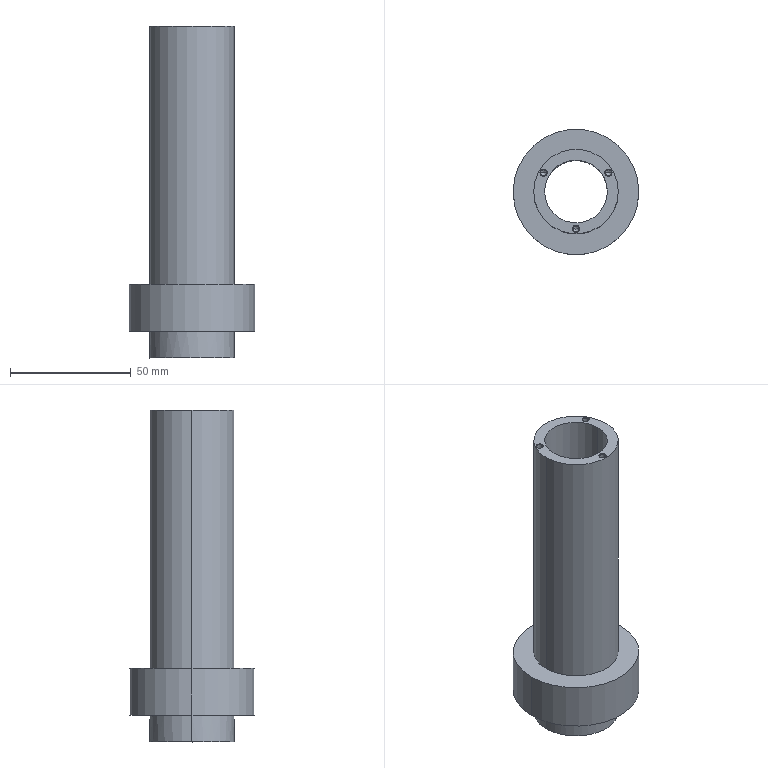Part | SolidWorks | features BaseBody 1 | 1 solid | 48 faces | box 52 x 52 x 137.45 mm | volume 81504 mm3 | cone 24 | cylinder 20 | plane 4 | commonest cylinder face diameters 2.5 x12 35 x4 26 x2 52 x2
STEP:
#1=CARTESIAN_POINT('',(359.676,258.457,27.673));
#2=VERTEX_POINT('',#1);
#3=CARTESIAN_POINT('',(360.758,257.832,26.922));
#4=VERTEX_POINT('',#3);
#5=CARTESIAN_POINT('',(360.287,258.104,27.249));
#6=DIRECTION('',(0.7423,-0.4286,-0.515));
#7=VECTOR('',#6,1000.);
#8=LINE('',#5,#7);
#9=EDGE_CURVE('',#2,#4,#8,.T.);
#10=ORIENTED_EDGE('',*,*,#9,.F.);
#11=CARTESIAN_POINT('',(358.593,259.082,26.922));
#12=VERTEX_POINT('',#11);
#13=CARTESIAN_POINT('',(359.065,258.81,27.249));
#14=DIRECTION('',(-0.7423,0.4286,-0.515));
#15=VECTOR('',#14,1000.);
#16=LINE('',#13,#15);
#17=EDGE_CURVE('',#2,#12,#16,.T.);
#18=ORIENTED_EDGE('',*,*,#17,.T.);
#19=CARTESIAN_POINT('',(359.676,258.457,26.922));
#20=DIRECTION('',(0.,0.,-1.));
#21=DIRECTION('',(0.866,-0.5,0.));
#22=AXIS2_PLACEMENT_3D('',#19,#20,#21);
#23=CIRCLE('',#22,1.25);
#24=EDGE_CURVE('',#12,#4,#23,.T.);
#25=ORIENTED_EDGE('',*,*,#24,.T.);
#26=EDGE_LOOP('',(#10,#18,#25));
#27=FACE_OUTER_BOUND('',#26,.T.);
#28=CARTESIAN_POINT('',(359.676,258.457,27.249));
#29=DIRECTION('',(0.,0.,-1.));
#30=DIRECTION('',(0.866,-0.5,0.));
#31=AXIS2_PLACEMENT_3D('',#28,#29,#30);
#32=CONICAL_SURFACE('',#31,0.7052,1.03);
#33=ADVANCED_FACE('',(#27),#32,.F.);
#34=CARTESIAN_POINT('',(360.758,257.832,15.721));
#35=VERTEX_POINT('',#34);
#36=CARTESIAN_POINT('',(360.301,259.54,15.721));
#37=VERTEX_POINT('',#36);
#38=CARTESIAN_POINT('',(359.676,258.457,15.721));
#39=DIRECTION('',(0.,0.,1.));
#40=DIRECTION('',(-0.866,0.5,0.));
#41=AXIS2_PLACEMENT_3D('',#38,#39,#40);
#42=CIRCLE('',#41,1.25);
#43=EDGE_CURVE('',#35,#37,#42,.T.);
#44=ORIENTED_EDGE('',*,*,#43,.F.);
#45=CARTESIAN_POINT('',(360.758,257.832,15.471));
#46=DIRECTION('',(0.,0.,1.));
#47=VECTOR('',#46,1000.);
#48=LINE('',#45,#47);
#49=EDGE_CURVE('',#35,#4,#48,.T.);
#50=ORIENTED_EDGE('',*,*,#49,.T.);
#51=ORIENTED_EDGE('',*,*,#24,.F.);
#52=CARTESIAN_POINT('',(358.593,259.082,15.721));
#53=VERTEX_POINT('',#52);
#54=CARTESIAN_POINT('',(358.593,259.082,15.471));
#55=DIRECTION('',(0.,0.,1.));
#56=VECTOR('',#55,1000.);
#57=LINE('',#54,#56);
#58=EDGE_CURVE('',#53,#12,#57,.T.);
#59=ORIENTED_EDGE('',*,*,#58,.F.);
#60=CARTESIAN_POINT('',(359.676,258.457,15.721));
#61=DIRECTION('',(0.,0.,1.));
#62=DIRECTION('',(-0.866,0.5,0.));
#63=AXIS2_PLACEMENT_3D('',#60,#61,#62);
#64=CIRCLE('',#63,1.25);
#65=EDGE_CURVE('',#37,#53,#64,.T.);
#66=ORIENTED_EDGE('',*,*,#65,.F.);
#67=EDGE_LOOP('',(#44,#50,#51,#59,#66));
#68=FACE_OUTER_BOUND('',#67,.T.);
#69=CARTESIAN_POINT('',(359.676,258.457,15.471));
#70=DIRECTION('',(0.,0.,1.));
#71=DIRECTION('',(-0.866,0.5,0.));
#72=AXIS2_PLACEMENT_3D('',#69,#70,#71);
#73=CYLINDRICAL_SURFACE('',#72,1.25);
#74=ADVANCED_FACE('',(#68),#73,.F.);
#75=ORIENTED_EDGE('',*,*,#65,.T.);
#76=CARTESIAN_POINT('',(359.051,257.375,15.721));
#77=VERTEX_POINT('',#76);
#78=CARTESIAN_POINT('',(359.676,258.457,15.721));
#79=DIRECTION('',(0.,0.,1.));
#80=DIRECTION('',(-0.866,0.5,0.));
#81=AXIS2_PLACEMENT_3D('',#78,#79,#80);
#82=CIRCLE('',#81,1.25);
#83=EDGE_CURVE('',#53,#77,#82,.T.);
#84=ORIENTED_EDGE('',*,*,#83,.T.);
#85=CARTESIAN_POINT('',(358.926,257.158,15.471));
#86=VERTEX_POINT('',#85);
#87=CARTESIAN_POINT('',(358.988,257.266,15.596));
#88=DIRECTION('',(-0.3536,-0.6124,-0.7071));
#89=VECTOR('',#88,1000.);
#90=LINE('',#87,#89);
#91=EDGE_CURVE('',#77,#86,#90,.T.);
#92=ORIENTED_EDGE('',*,*,#91,.T.);
#93=CARTESIAN_POINT('',(360.426,259.756,15.471));
#94=VERTEX_POINT('',#93);
#95=CARTESIAN_POINT('',(359.676,258.457,15.471));
#96=DIRECTION('',(0.,0.,1.));
#97=DIRECTION('',(0.866,-0.5,0.));
#98=AXIS2_PLACEMENT_3D('',#95,#96,#97);
#99=CIRCLE('',#98,1.5);
#100=EDGE_CURVE('',#94,#86,#99,.T.);
#101=ORIENTED_EDGE('',*,*,#100,.F.);
#102=CARTESIAN_POINT('',(360.363,259.648,15.596));
#103=DIRECTION('',(0.3536,0.6124,-0.7071));
#104=VECTOR('',#103,1000.);
#105=LINE('',#102,#104);
#106=EDGE_CURVE('',#37,#94,#105,.T.);
#107=ORIENTED_EDGE('',*,*,#106,.F.);
#108=EDGE_LOOP('',(#75,#84,#92,#101,#107));
#109=FACE_OUTER_BOUND('',#108,.T.);
#110=CARTESIAN_POINT('',(359.676,258.457,15.596));
#111=DIRECTION('',(0.,0.,-1.));
#112=DIRECTION('',(0.5,0.866,0.));
#113=AXIS2_PLACEMENT_3D('',#110,#111,#112);
#114=CONICAL_SURFACE('',#113,1.375,0.7854);
#115=ADVANCED_FACE('',(#109),#114,.F.);
#116=CARTESIAN_POINT('',(322.653,258.943,15.721));
#117=VERTEX_POINT('',#116);
#118=CARTESIAN_POINT('',(320.946,259.401,15.721));
#119=VERTEX_POINT('',#118);
#120=CARTESIAN_POINT('',(321.571,258.318,15.721));
#121=DIRECTION('',(0.,0.,1.));
#122=DIRECTION('',(-0.866,-0.5,0.));
#123=AXIS2_PLACEMENT_3D('',#120,#121,#122);
#124=CIRCLE('',#123,1.25);
#125=EDGE_CURVE('',#117,#119,#124,.T.);
#126=ORIENTED_EDGE('',*,*,#125,.T.);
#127=CARTESIAN_POINT('',(320.821,259.617,15.471));
#128=VERTEX_POINT('',#127);
#129=CARTESIAN_POINT('',(320.883,259.509,15.596));
#130=DIRECTION('',(-0.3536,0.6124,-0.7071));
#131=VECTOR('',#130,1000.);
#132=LINE('',#129,#131);
#133=EDGE_CURVE('',#119,#128,#132,.T.);
#134=ORIENTED_EDGE('',*,*,#133,.T.);
#135=CARTESIAN_POINT('',(322.321,257.019,15.471));
#136=VERTEX_POINT('',#135);
#137=CARTESIAN_POINT('',(321.571,258.318,15.471));
#138=DIRECTION('',(0.,0.,1.));
#139=DIRECTION('',(0.5,-0.866,0.));
#140=AXIS2_PLACEMENT_3D('',#137,#138,#139);
#141=CIRCLE('',#140,1.5);
#142=EDGE_CURVE('',#136,#128,#141,.T.);
#143=ORIENTED_EDGE('',*,*,#142,.F.);
#144=CARTESIAN_POINT('',(322.196,257.236,15.721));
#145=VERTEX_POINT('',#144);
#146=CARTESIAN_POINT('',(322.258,257.128,15.596));
#147=DIRECTION('',(0.3536,-0.6124,-0.7071));
#148=VECTOR('',#147,1000.);
#149=LINE('',#146,#148);
#150=EDGE_CURVE('',#145,#136,#149,.T.);
#151=ORIENTED_EDGE('',*,*,#150,.F.);
#152=CARTESIAN_POINT('',(321.571,258.318,15.721));
#153=DIRECTION('',(0.,0.,1.));
#154=DIRECTION('',(-0.866,-0.5,0.));
#155=AXIS2_PLACEMENT_3D('',#152,#153,#154);
#156=CIRCLE('',#155,1.25);
#157=EDGE_CURVE('',#145,#117,#156,.T.);
#158=ORIENTED_EDGE('',*,*,#157,.T.);
#159=EDGE_LOOP('',(#126,#134,#143,#151,#158));
#160=FACE_OUTER_BOUND('',#159,.T.);
#161=CARTESIAN_POINT('',(321.571,258.318,15.596));
#162=DIRECTION('',(0.,0.,-1.));
#163=DIRECTION('',(0.5,-0.866,0.));
#164=AXIS2_PLACEMENT_3D('',#161,#162,#163);
#165=CONICAL_SURFACE('',#164,1.375,0.7854);
#166=ADVANCED_FACE('',(#160),#165,.F.);
#167=CARTESIAN_POINT('',(320.488,257.693,15.721));
#168=VERTEX_POINT('',#167);
#169=CARTESIAN_POINT('',(321.571,258.318,15.721));
#170=DIRECTION('',(0.,0.,1.));
#171=DIRECTION('',(-0.866,-0.5,0.));
#172=AXIS2_PLACEMENT_3D('',#169,#170,#171);
#173=CIRCLE('',#172,1.25);
#174=EDGE_CURVE('',#168,#145,#173,.T.);
#175=ORIENTED_EDGE('',*,*,#174,.F.);
#176=CARTESIAN_POINT('',(320.488,257.693,26.922));
#177=VERTEX_POINT('',#176);
#178=CARTESIAN_POINT('',(320.488,257.693,15.471));
#179=DIRECTION('',(0.,0.,1.));
#180=VECTOR('',#179,1000.);
#181=LINE('',#178,#180);
#182=EDGE_CURVE('',#168,#177,#181,.T.);
#183=ORIENTED_EDGE('',*,*,#182,.T.);
#184=CARTESIAN_POINT('',(322.653,258.943,26.922));
#185=VERTEX_POINT('',#184);
#186=CARTESIAN_POINT('',(321.571,258.318,26.922));
#187=DIRECTION('',(0.,0.,-1.));
#188=DIRECTION('',(-0.866,-0.5,0.));
#189=AXIS2_PLACEMENT_3D('',#186,#187,#188);
#190=CIRCLE('',#189,1.25);
#191=EDGE_CURVE('',#185,#177,#190,.T.);
#192=ORIENTED_EDGE('',*,*,#191,.F.);
#193=CARTESIAN_POINT('',(322.653,258.943,15.471));
#194=DIRECTION('',(0.,0.,1.));
#195=VECTOR('',#194,1000.);
#196=LINE('',#193,#195);
#197=EDGE_CURVE('',#117,#185,#196,.T.);
#198=ORIENTED_EDGE('',*,*,#197,.F.);
#199=ORIENTED_EDGE('',*,*,#157,.F.);
#200=EDGE_LOOP('',(#175,#183,#192,#198,#199));
#201=FACE_OUTER_BOUND('',#200,.T.);
#202=CARTESIAN_POINT('',(321.571,258.318,15.471));
#203=DIRECTION('',(0.,0.,1.));
#204=DIRECTION('',(0.866,0.5,0.));
#205=AXIS2_PLACEMENT_3D('',#202,#203,#204);
#206=CYLINDRICAL_SURFACE('',#205,1.25);
#207=ADVANCED_FACE('',(#201),#206,.F.);
#208=CARTESIAN_POINT('',(321.571,258.318,27.673));
#209=VERTEX_POINT('',#208);
#210=CARTESIAN_POINT('',(320.96,257.966,27.249));
#211=DIRECTION('',(-0.7423,-0.4286,-0.515));
#212=VECTOR('',#211,1000.);
#213=LINE('',#210,#212);
#214=EDGE_CURVE('',#209,#177,#213,.T.);
#215=ORIENTED_EDGE('',*,*,#214,.F.);
#216=CARTESIAN_POINT('',(322.182,258.671,27.249));
#217=DIRECTION('',(0.7423,0.4286,-0.515));
#218=VECTOR('',#217,1000.);
#219=LINE('',#216,#218);
#220=EDGE_CURVE('',#209,#185,#219,.T.);
#221=ORIENTED_EDGE('',*,*,#220,.T.);
#222=ORIENTED_EDGE('',*,*,#191,.T.);
#223=EDGE_LOOP('',(#215,#221,#222));
#224=FACE_OUTER_BOUND('',#223,.T.);
#225=CARTESIAN_POINT('',(321.571,258.318,27.249));
#226=DIRECTION('',(0.,0.,-1.));
#227=DIRECTION('',(-0.866,-0.5,0.));
#228=AXIS2_PLACEMENT_3D('',#225,#226,#227);
#229=CONICAL_SURFACE('',#228,0.7052,1.03);
#230=ADVANCED_FACE('',(#224),#229,.F.);
#231=CARTESIAN_POINT('',(340.503,290.138,15.721));
#232=VERTEX_POINT('',#231);
#233=CARTESIAN_POINT('',(341.753,291.388,15.721));
#234=VERTEX_POINT('',#233);
#235=CARTESIAN_POINT('',(340.503,291.388,15.721));
#236=DIRECTION('',(0.,0.,1.));
#237=DIRECTION('',(0.,1.,0.));
#238=AXIS2_PLACEMENT_3D('',#235,#236,#237);
#239=CIRCLE('',#238,1.25);
#240=EDGE_CURVE('',#232,#234,#239,.T.);
#241=ORIENTED_EDGE('',*,*,#240,.T.);
#242=CARTESIAN_POINT('',(342.003,291.388,15.471));
#243=VERTEX_POINT('',#242);
#244=CARTESIAN_POINT('',(341.878,291.388,15.596));
#245=DIRECTION('',(0.7071,0.,-0.7071));
#246=VECTOR('',#245,1000.);
#247=LINE('',#244,#246);
#248=EDGE_CURVE('',#234,#243,#247,.T.);
#249=ORIENTED_EDGE('',*,*,#248,.T.);
#250=CARTESIAN_POINT('',(339.003,291.388,15.471));
#251=VERTEX_POINT('',#250);
#252=CARTESIAN_POINT('',(340.503,291.388,15.471));
#253=DIRECTION('',(0.,0.,1.));
#254=DIRECTION('',(-1.,0.,0.));
#255=AXIS2_PLACEMENT_3D('',#252,#253,#254);
#256=CIRCLE('',#255,1.5);
#257=EDGE_CURVE('',#251,#243,#256,.T.);
#258=ORIENTED_EDGE('',*,*,#257,.F.);
#259=CARTESIAN_POINT('',(339.253,291.388,15.721));
#260=VERTEX_POINT('',#259);
#261=CARTESIAN_POINT('',(339.128,291.388,15.596));
#262=DIRECTION('',(-0.7071,0.,-0.7071));
#263=VECTOR('',#262,1000.);
#264=LINE('',#261,#263);
#265=EDGE_CURVE('',#260,#251,#264,.T.);
#266=ORIENTED_EDGE('',*,*,#265,.F.);
#267=CARTESIAN_POINT('',(340.503,291.388,15.721));
#268=DIRECTION('',(0.,0.,1.));
#269=DIRECTION('',(0.,1.,0.));
#270=AXIS2_PLACEMENT_3D('',#267,#268,#269);
#271=CIRCLE('',#270,1.25);
#272=EDGE_CURVE('',#260,#232,#271,.T.);
#273=ORIENTED_EDGE('',*,*,#272,.T.);
#274=EDGE_LOOP('',(#241,#249,#258,#266,#273));
#275=FACE_OUTER_BOUND('',#274,.T.);
#276=CARTESIAN_POINT('',(340.503,291.388,15.596));
#277=DIRECTION('',(0.,0.,-1.));
#278=DIRECTION('',(-1.,0.,0.));
#279=AXIS2_PLACEMENT_3D('',#276,#277,#278);
#280=CONICAL_SURFACE('',#279,1.375,0.7854);
#281=ADVANCED_FACE('',(#275),#280,.F.);
#282=CARTESIAN_POINT('',(340.503,292.638,15.721));
#283=VERTEX_POINT('',#282);
#284=CARTESIAN_POINT('',(340.503,291.388,15.721));
#285=DIRECTION('',(0.,0.,1.));
#286=DIRECTION('',(0.,1.,0.));
#287=AXIS2_PLACEMENT_3D('',#284,#285,#286);
#288=CIRCLE('',#287,1.25);
#289=EDGE_CURVE('',#283,#260,#288,.T.);
#290=ORIENTED_EDGE('',*,*,#289,.F.);
#291=CARTESIAN_POINT('',(340.503,292.638,26.922));
#292=VERTEX_POINT('',#291);
#293=CARTESIAN_POINT('',(340.503,292.638,15.471));
#294=DIRECTION('',(0.,0.,1.));
#295=VECTOR('',#294,1000.);
#296=LINE('',#293,#295);
#297=EDGE_CURVE('',#283,#292,#296,.T.);
#298=ORIENTED_EDGE('',*,*,#297,.T.);
#299=CARTESIAN_POINT('',(340.503,290.138,26.922));
#300=VERTEX_POINT('',#299);
#301=CARTESIAN_POINT('',(340.503,291.388,26.922));
#302=DIRECTION('',(0.,0.,-1.));
#303=DIRECTION('',(0.,1.,0.));
#304=AXIS2_PLACEMENT_3D('',#301,#302,#303);
#305=CIRCLE('',#304,1.25);
#306=EDGE_CURVE('',#300,#292,#305,.T.);
#307=ORIENTED_EDGE('',*,*,#306,.F.);
#308=CARTESIAN_POINT('',(340.503,290.138,15.471));
#309=DIRECTION('',(0.,0.,1.));
#310=VECTOR('',#309,1000.);
#311=LINE('',#308,#310);
#312=EDGE_CURVE('',#232,#300,#311,.T.);
#313=ORIENTED_EDGE('',*,*,#312,.F.);
#314=ORIENTED_EDGE('',*,*,#272,.F.);
#315=EDGE_LOOP('',(#290,#298,#307,#313,#314));
#316=FACE_OUTER_BOUND('',#315,.T.);
#317=CARTESIAN_POINT('',(340.503,291.388,15.471));
#318=DIRECTION('',(0.,0.,1.));
#319=DIRECTION('',(0.,-1.,0.));
#320=AXIS2_PLACEMENT_3D('',#317,#318,#319);
#321=CYLINDRICAL_SURFACE('',#320,1.25);
#322=ADVANCED_FACE('',(#316),#321,.F.);
#323=CARTESIAN_POINT('',(340.503,291.388,27.673));
#324=VERTEX_POINT('',#323);
#325=CARTESIAN_POINT('',(340.503,292.093,27.249));
#326=DIRECTION('',(0.,0.8572,-0.515));
#327=VECTOR('',#326,1000.);
#328=LINE('',#325,#327);
#329=EDGE_CURVE('',#324,#292,#328,.T.);
#330=ORIENTED_EDGE('',*,*,#329,.F.);
#331=CARTESIAN_POINT('',(340.503,290.682,27.249));
#332=DIRECTION('',(0.,-0.8572,-0.515));
#333=VECTOR('',#332,1000.);
#334=LINE('',#331,#333);
#335=EDGE_CURVE('',#324,#300,#334,.T.);
#336=ORIENTED_EDGE('',*,*,#335,.T.);
#337=ORIENTED_EDGE('',*,*,#306,.T.);
#338=EDGE_LOOP('',(#330,#336,#337));
#339=FACE_OUTER_BOUND('',#338,.T.);
#340=CARTESIAN_POINT('',(340.503,291.388,27.249));
#341=DIRECTION('',(0.,0.,-1.));
#342=DIRECTION('',(0.,1.,0.));
#343=AXIS2_PLACEMENT_3D('',#340,#341,#342);
#344=CONICAL_SURFACE('',#343,0.7052,1.03);
#345=ADVANCED_FACE('',(#339),#344,.F.);
#346=CARTESIAN_POINT('',(314.583,269.388,34.922));
#347=VERTEX_POINT('',#346);
#348=CARTESIAN_POINT('',(366.583,269.388,34.922));
#349=VERTEX_POINT('',#348);
#350=CARTESIAN_POINT('',(340.583,269.388,34.922));
#351=DIRECTION('',(0.,0.,1.));
#352=DIRECTION('',(-1.,0.,0.));
#353=AXIS2_PLACEMENT_3D('',#350,#351,#352);
#354=CIRCLE('',#353,26.);
#355=EDGE_CURVE('',#347,#349,#354,.T.);
#356=ORIENTED_EDGE('',*,*,#355,.F.);
#357=CARTESIAN_POINT('',(314.583,269.388,15.471));
#358=VERTEX_POINT('',#357);
#359=CARTESIAN_POINT('',(314.583,269.388,35.471));
#360=DIRECTION('',(0.,0.,-1.));
#361=VECTOR('',#360,1000.);
#362=LINE('',#359,#361);
#363=EDGE_CURVE('',#347,#358,#362,.T.);
#364=ORIENTED_EDGE('',*,*,#363,.T.);
#365=CARTESIAN_POINT('',(366.583,269.388,15.471));
#366=VERTEX_POINT('',#365);
#367=CARTESIAN_POINT('',(340.583,269.388,15.471));
#368=DIRECTION('',(0.,0.,-1.));
#369=DIRECTION('',(-1.,0.,0.));
#370=AXIS2_PLACEMENT_3D('',#367,#368,#369);
#371=CIRCLE('',#370,26.);
#372=EDGE_CURVE('',#366,#358,#371,.T.);
#373=ORIENTED_EDGE('',*,*,#372,.F.);
#374=CARTESIAN_POINT('',(366.583,269.388,35.471));
#375=DIRECTION('',(0.,0.,-1.));
#376=VECTOR('',#375,1000.);
#377=LINE('',#374,#376);
#378=EDGE_CURVE('',#349,#366,#377,.T.);
#379=ORIENTED_EDGE('',*,*,#378,.F.);
#380=EDGE_LOOP('',(#356,#364,#373,#379));
#381=FACE_OUTER_BOUND('',#380,.T.);
#382=CARTESIAN_POINT('',(340.583,269.388,35.471));
#383=DIRECTION('',(0.,0.,-1.));
#384=DIRECTION('',(1.,0.,0.));
#385=AXIS2_PLACEMENT_3D('',#382,#383,#384);
#386=CYLINDRICAL_SURFACE('',#385,26.);
#387=ADVANCED_FACE('',(#381),#386,.T.);
#388=CARTESIAN_POINT('',(358.083,269.388,141.922));
#389=VERTEX_POINT('',#388);
#390=CARTESIAN_POINT('',(323.083,269.388,141.922));
#391=VERTEX_POINT('',#390);
#392=CARTESIAN_POINT('',(340.583,269.388,141.922));
#393=DIRECTION('',(0.,0.,1.));
#394=DIRECTION('',(-1.,0.,0.));
#395=AXIS2_PLACEMENT_3D('',#392,#393,#394);
#396=CIRCLE('',#395,17.5);
#397=EDGE_CURVE('',#389,#391,#396,.T.);
#398=ORIENTED_EDGE('',*,*,#397,.F.);
#399=CARTESIAN_POINT('',(358.083,269.388,34.922));
#400=VERTEX_POINT('',#399);
#401=CARTESIAN_POINT('',(358.083,269.388,-6.009));
#402=DIRECTION('',(0.,0.,-1.));
#403=VECTOR('',#402,1000.);
#404=LINE('',#401,#403);
#405=EDGE_CURVE('',#389,#400,#404,.T.);
#406=ORIENTED_EDGE('',*,*,#405,.T.);
#407=CARTESIAN_POINT('',(323.083,269.388,34.922));
#408=VERTEX_POINT('',#407);
#409=CARTESIAN_POINT('',(340.583,269.388,34.922));
#410=DIRECTION('',(0.,0.,-1.));
#411=DIRECTION('',(-1.,0.000000007,0.));
#412=AXIS2_PLACEMENT_3D('',#409,#410,#411);
#413=CIRCLE('',#412,17.5);
#414=EDGE_CURVE('',#408,#400,#413,.T.);
#415=ORIENTED_EDGE('',*,*,#414,.F.);
#416=CARTESIAN_POINT('',(323.083,269.388,-6.009));
#417=DIRECTION('',(0.,0.,-1.));
#418=VECTOR('',#417,1000.);
#419=LINE('',#416,#418);
#420=EDGE_CURVE('',#391,#408,#419,.T.);
#421=ORIENTED_EDGE('',*,*,#420,.F.);
#422=EDGE_LOOP('',(#398,#406,#415,#421));
#423=FACE_OUTER_BOUND('',#422,.T.);
#424=CARTESIAN_POINT('',(340.583,269.388,-6.009));
#425=DIRECTION('',(0.,0.,-1.));
#426=DIRECTION('',(-1.,0.000000007,0.));
#427=AXIS2_PLACEMENT_3D('',#424,#425,#426);
#428=CYLINDRICAL_SURFACE('',#427,17.5);
#429=ADVANCED_FACE('',(#423),#428,.T.);
#430=CARTESIAN_POINT('',(341.833,253.888,141.672));
#431=VERTEX_POINT('',#430);
#432=CARTESIAN_POINT('',(339.333,253.888,141.672));
#433=VERTEX_POINT('',#432);
#434=CARTESIAN_POINT('',(340.583,253.888,141.672));
#435=DIRECTION('',(0.,0.,-1.));
#436=DIRECTION('',(-1.,0.,0.));
#437=AXIS2_PLACEMENT_3D('',#434,#435,#436);
#438=CIRCLE('',#437,1.25);
#439=EDGE_CURVE('',#431,#433,#438,.T.);
#440=ORIENTED_EDGE('',*,*,#439,.T.);
#441=CARTESIAN_POINT('',(339.083,253.888,141.922));
#442=VERTEX_POINT('',#441);
#443=CARTESIAN_POINT('',(339.208,253.888,141.797));
#444=DIRECTION('',(-0.7071,0.,0.7071));
#445=VECTOR('',#444,1000.);
#446=LINE('',#443,#445);
#447=EDGE_CURVE('',#433,#442,#446,.T.);
#448=ORIENTED_EDGE('',*,*,#447,.T.);
#449=CARTESIAN_POINT('',(342.083,253.888,141.922));
#450=VERTEX_POINT('',#449);
#451=CARTESIAN_POINT('',(340.583,253.888,141.922));
#452=DIRECTION('',(0.,0.,-1.));
#453=DIRECTION('',(1.,0.,0.));
#454=AXIS2_PLACEMENT_3D('',#451,#452,#453);
#455=CIRCLE('',#454,1.5);
#456=EDGE_CURVE('',#450,#442,#455,.T.);
#457=ORIENTED_EDGE('',*,*,#456,.F.);
#458=CARTESIAN_POINT('',(341.958,253.888,141.797));
#459=DIRECTION('',(0.7071,0.,0.7071));
#460=VECTOR('',#459,1000.);
#461=LINE('',#458,#460);
#462=EDGE_CURVE('',#431,#450,#461,.T.);
#463=ORIENTED_EDGE('',*,*,#462,.F.);
#464=EDGE_LOOP('',(#440,#448,#457,#463));
#465=FACE_OUTER_BOUND('',#464,.T.);
#466=CARTESIAN_POINT('',(340.583,253.888,141.797));
#467=DIRECTION('',(0.,0.,1.));
#468=DIRECTION('',(1.,0.,0.));
#469=AXIS2_PLACEMENT_3D('',#466,#467,#468);
#470=CONICAL_SURFACE('',#469,1.375,0.7854);
#471=ADVANCED_FACE('',(#465),#470,.F.);
#472=ORIENTED_EDGE('',*,*,#439,.F.);
#473=CARTESIAN_POINT('',(341.833,253.888,129.922));
#474=VERTEX_POINT('',#473);
#475=CARTESIAN_POINT('',(341.833,253.888,141.922));
#476=DIRECTION('',(0.,0.,-1.));
#477=VECTOR('',#476,1000.);
#478=LINE('',#475,#477);
#479=EDGE_CURVE('',#431,#474,#478,.T.);
#480=ORIENTED_EDGE('',*,*,#479,.T.);
#481=CARTESIAN_POINT('',(339.333,253.888,129.922));
#482=VERTEX_POINT('',#481);
#483=CARTESIAN_POINT('',(340.583,253.888,129.922));
#484=DIRECTION('',(0.,0.,1.));
#485=DIRECTION('',(1.,0.,0.));
#486=AXIS2_PLACEMENT_3D('',#483,#484,#485);
#487=CIRCLE('',#486,1.25);
#488=EDGE_CURVE('',#482,#474,#487,.T.);
#489=ORIENTED_EDGE('',*,*,#488,.F.);
#490=CARTESIAN_POINT('',(339.333,253.888,141.922));
#491=DIRECTION('',(0.,0.,-1.));
#492=VECTOR('',#491,1000.);
#493=LINE('',#490,#492);
#494=EDGE_CURVE('',#433,#482,#493,.T.);
#495=ORIENTED_EDGE('',*,*,#494,.F.);
#496=EDGE_LOOP('',(#472,#480,#489,#495));
#497=FACE_OUTER_BOUND('',#496,.T.);
#498=CARTESIAN_POINT('',(340.583,253.888,141.922));
#499=DIRECTION('',(0.,0.,-1.));
#500=DIRECTION('',(-1.,0.,0.));
#501=AXIS2_PLACEMENT_3D('',#498,#499,#500);
#502=CYLINDRICAL_SURFACE('',#501,1.25);
#503=ADVANCED_FACE('',(#497),#502,.F.);
#504=CARTESIAN_POINT('',(340.583,253.888,129.171));
#505=VERTEX_POINT('',#504);
#506=CARTESIAN_POINT('',(341.289,253.888,129.595));
#507=DIRECTION('',(0.8572,0.,0.515));
#508=VECTOR('',#507,1000.);
#509=LINE('',#506,#508);
#510=EDGE_CURVE('',#505,#474,#509,.T.);
#511=ORIENTED_EDGE('',*,*,#510,.F.);
#512=CARTESIAN_POINT('',(339.878,253.888,129.595));
#513=DIRECTION('',(-0.8572,0.,0.515));
#514=VECTOR('',#513,1000.);
#515=LINE('',#512,#514);
#516=EDGE_CURVE('',#505,#482,#515,.T.);
#517=ORIENTED_EDGE('',*,*,#516,.T.);
#518=ORIENTED_EDGE('',*,*,#488,.T.);
#519=EDGE_LOOP('',(#511,#517,#518));
#520=FACE_OUTER_BOUND('',#519,.T.);
#521=CARTESIAN_POINT('',(340.583,253.888,129.595));
#522=DIRECTION('',(0.,0.,1.));
#523=DIRECTION('',(1.,0.,0.));
#524=AXIS2_PLACEMENT_3D('',#521,#522,#523);
#525=CONICAL_SURFACE('',#524,0.7052,1.03);
#526=ADVANCED_FACE('',(#520),#525,.F.);
#527=CARTESIAN_POINT('',(355.257,277.138,141.672));
#528=VERTEX_POINT('',#527);
#529=CARTESIAN_POINT('',(352.757,277.138,141.672));
#530=VERTEX_POINT('',#529);
#531=CARTESIAN_POINT('',(354.007,277.138,141.672));
#532=DIRECTION('',(0.,0.,-1.));
#533=DIRECTION('',(-1.,0.,0.));
#534=AXIS2_PLACEMENT_3D('',#531,#532,#533);
#535=CIRCLE('',#534,1.25);
#536=EDGE_CURVE('',#528,#530,#535,.T.);
#537=ORIENTED_EDGE('',*,*,#536,.T.);
#538=CARTESIAN_POINT('',(352.507,277.138,141.922));
#539=VERTEX_POINT('',#538);
#540=CARTESIAN_POINT('',(352.632,277.138,141.797));
#541=DIRECTION('',(-0.7071,0.,0.7071));
#542=VECTOR('',#541,1000.);
#543=LINE('',#540,#542);
#544=EDGE_CURVE('',#530,#539,#543,.T.);
#545=ORIENTED_EDGE('',*,*,#544,.T.);
#546=CARTESIAN_POINT('',(355.507,277.138,141.922));
#547=VERTEX_POINT('',#546);
#548=CARTESIAN_POINT('',(354.007,277.138,141.922));
#549=DIRECTION('',(0.,0.,-1.));
#550=DIRECTION('',(1.,0.,0.));
#551=AXIS2_PLACEMENT_3D('',#548,#549,#550);
#552=CIRCLE('',#551,1.5);
#553=EDGE_CURVE('',#547,#539,#552,.T.);
#554=ORIENTED_EDGE('',*,*,#553,.F.);
#555=CARTESIAN_POINT('',(355.382,277.138,141.797));
#556=DIRECTION('',(0.7071,0.,0.7071));
#557=VECTOR('',#556,1000.);
#558=LINE('',#555,#557);
#559=EDGE_CURVE('',#528,#547,#558,.T.);
#560=ORIENTED_EDGE('',*,*,#559,.F.);
#561=EDGE_LOOP('',(#537,#545,#554,#560));
#562=FACE_OUTER_BOUND('',#561,.T.);
#563=CARTESIAN_POINT('',(354.007,277.138,141.797));
#564=DIRECTION('',(0.,0.,1.));
#565=DIRECTION('',(1.,0.,0.));
#566=AXIS2_PLACEMENT_3D('',#563,#564,#565);
#567=CONICAL_SURFACE('',#566,1.375,0.7854);
#568=ADVANCED_FACE('',(#562),#567,.F.);
#569=ORIENTED_EDGE('',*,*,#536,.F.);
#570=CARTESIAN_POINT('',(355.257,277.138,129.922));
#571=VERTEX_POINT('',#570);
#572=CARTESIAN_POINT('',(355.257,277.138,141.922));
#573=DIRECTION('',(0.,0.,-1.));
#574=VECTOR('',#573,1000.);
#575=LINE('',#572,#574);
#576=EDGE_CURVE('',#528,#571,#575,.T.);
#577=ORIENTED_EDGE('',*,*,#576,.T.);
#578=CARTESIAN_POINT('',(352.757,277.138,129.922));
#579=VERTEX_POINT('',#578);
#580=CARTESIAN_POINT('',(354.007,277.138,129.922));
#581=DIRECTION('',(0.,0.,1.));
#582=DIRECTION('',(1.,0.,0.));
#583=AXIS2_PLACEMENT_3D('',#580,#581,#582);
#584=CIRCLE('',#583,1.25);
#585=EDGE_CURVE('',#579,#571,#584,.T.);
#586=ORIENTED_EDGE('',*,*,#585,.F.);
#587=CARTESIAN_POINT('',(352.757,277.138,141.922));
#588=DIRECTION('',(0.,0.,-1.));
#589=VECTOR('',#588,1000.);
#590=LINE('',#587,#589);
#591=EDGE_CURVE('',#530,#579,#590,.T.);
#592=ORIENTED_EDGE('',*,*,#591,.F.);
#593=EDGE_LOOP('',(#569,#577,#586,#592));
#594=FACE_OUTER_BOUND('',#593,.T.);
#595=CARTESIAN_POINT('',(354.007,277.138,141.922));
#596=DIRECTION('',(0.,0.,-1.));
#597=DIRECTION('',(-1.,0.,0.));
#598=AXIS2_PLACEMENT_3D('',#595,#596,#597);
#599=CYLINDRICAL_SURFACE('',#598,1.25);
#600=ADVANCED_FACE('',(#594),#599,.F.);
#601=CARTESIAN_POINT('',(354.007,277.138,129.171));
#602=VERTEX_POINT('',#601);
#603=CARTESIAN_POINT('',(354.712,277.138,129.595));
#604=DIRECTION('',(0.8572,0.,0.515));
#605=VECTOR('',#604,1000.);
#606=LINE('',#603,#605);
#607=EDGE_CURVE('',#602,#571,#606,.T.);
#608=ORIENTED_EDGE('',*,*,#607,.F.);
#609=CARTESIAN_POINT('',(353.302,277.138,129.595));
#610=DIRECTION('',(-0.8572,0.,0.515));
#611=VECTOR('',#610,1000.);
#612=LINE('',#609,#611);
#613=EDGE_CURVE('',#602,#579,#612,.T.);
#614=ORIENTED_EDGE('',*,*,#613,.T.);
#615=ORIENTED_EDGE('',*,*,#585,.T.);
#616=EDGE_LOOP('',(#608,#614,#615));
#617=FACE_OUTER_BOUND('',#616,.T.);
#618=CARTESIAN_POINT('',(354.007,277.138,129.595));
#619=DIRECTION('',(0.,0.,1.));
#620=DIRECTION('',(1.,0.,0.));
#621=AXIS2_PLACEMENT_3D('',#618,#619,#620);
#622=CONICAL_SURFACE('',#621,0.7052,1.03);
#623=ADVANCED_FACE('',(#617),#622,.F.);
#624=CARTESIAN_POINT('',(328.41,277.138,141.672));
#625=VERTEX_POINT('',#624);
#626=CARTESIAN_POINT('',(325.91,277.138,141.672));
#627=VERTEX_POINT('',#626);
#628=CARTESIAN_POINT('',(327.16,277.138,141.672));
#629=DIRECTION('',(0.,0.,-1.));
#630=DIRECTION('',(-1.,0.,0.));
#631=AXIS2_PLACEMENT_3D('',#628,#629,#630);
#632=CIRCLE('',#631,1.25);
#633=EDGE_CURVE('',#625,#627,#632,.T.);
#634=ORIENTED_EDGE('',*,*,#633,.T.);
#635=CARTESIAN_POINT('',(325.66,277.138,141.922));
#636=VERTEX_POINT('',#635);
#637=CARTESIAN_POINT('',(325.785,277.138,141.797));
#638=DIRECTION('',(-0.7071,0.,0.7071));
#639=VECTOR('',#638,1000.);
#640=LINE('',#637,#639);
#641=EDGE_CURVE('',#627,#636,#640,.T.);
#642=ORIENTED_EDGE('',*,*,#641,.T.);
#643=CARTESIAN_POINT('',(328.66,277.138,141.922));
#644=VERTEX_POINT('',#643);
#645=CARTESIAN_POINT('',(327.16,277.138,141.922));
#646=DIRECTION('',(0.,0.,-1.));
#647=DIRECTION('',(1.,0.,0.));
#648=AXIS2_PLACEMENT_3D('',#645,#646,#647);
#649=CIRCLE('',#648,1.5);
#650=EDGE_CURVE('',#644,#636,#649,.T.);
#651=ORIENTED_EDGE('',*,*,#650,.F.);
#652=CARTESIAN_POINT('',(328.535,277.138,141.797));
#653=DIRECTION('',(0.7071,0.,0.7071));
#654=VECTOR('',#653,1000.);
#655=LINE('',#652,#654);
#656=EDGE_CURVE('',#625,#644,#655,.T.);
#657=ORIENTED_EDGE('',*,*,#656,.F.);
#658=EDGE_LOOP('',(#634,#642,#651,#657));
#659=FACE_OUTER_BOUND('',#658,.T.);
#660=CARTESIAN_POINT('',(327.16,277.138,141.797));
#661=DIRECTION('',(0.,0.,1.));
#662=DIRECTION('',(1.,0.,0.));
#663=AXIS2_PLACEMENT_3D('',#660,#661,#662);
#664=CONICAL_SURFACE('',#663,1.375,0.7854);
#665=ADVANCED_FACE('',(#659),#664,.F.);
#666=ORIENTED_EDGE('',*,*,#633,.F.);
#667=CARTESIAN_POINT('',(328.41,277.138,129.922));
#668=VERTEX_POINT('',#667);
#669=CARTESIAN_POINT('',(328.41,277.138,141.922));
#670=DIRECTION('',(0.,0.,-1.));
#671=VECTOR('',#670,1000.);
#672=LINE('',#669,#671);
#673=EDGE_CURVE('',#625,#668,#672,.T.);
#674=ORIENTED_EDGE('',*,*,#673,.T.);
#675=CARTESIAN_POINT('',(325.91,277.138,129.922));
#676=VERTEX_POINT('',#675);
#677=CARTESIAN_POINT('',(327.16,277.138,129.922));
#678=DIRECTION('',(0.,0.,1.));
#679=DIRECTION('',(1.,0.,0.));
#680=AXIS2_PLACEMENT_3D('',#677,#678,#679);
#681=CIRCLE('',#680,1.25);
#682=EDGE_CURVE('',#676,#668,#681,.T.);
#683=ORIENTED_EDGE('',*,*,#682,.F.);
#684=CARTESIAN_POINT('',(325.91,277.138,141.922));
#685=DIRECTION('',(0.,0.,-1.));
#686=VECTOR('',#685,1000.);
#687=LINE('',#684,#686);
#688=EDGE_CURVE('',#627,#676,#687,.T.);
#689=ORIENTED_EDGE('',*,*,#688,.F.);
#690=EDGE_LOOP('',(#666,#674,#683,#689));
#691=FACE_OUTER_BOUND('',#690,.T.);
#692=CARTESIAN_POINT('',(327.16,277.138,141.922));
#693=DIRECTION('',(0.,0.,-1.));
#694=DIRECTION('',(-1.,0.,0.));
#695=AXIS2_PLACEMENT_3D('',#692,#693,#694);
#696=CYLINDRICAL_SURFACE('',#695,1.25);
#697=ADVANCED_FACE('',(#691),#696,.F.);
#698=CARTESIAN_POINT('',(327.16,277.138,129.171));
#699=VERTEX_POINT('',#698);
#700=CARTESIAN_POINT('',(327.865,277.138,129.595));
#701=DIRECTION('',(0.8572,0.,0.515));
#702=VECTOR('',#701,1000.);
#703=LINE('',#700,#702);
#704=EDGE_CURVE('',#699,#668,#703,.T.);
#705=ORIENTED_EDGE('',*,*,#704,.F.);
#706=CARTESIAN_POINT('',(326.455,277.138,129.595));
#707=DIRECTION('',(-0.8572,0.,0.515));
#708=VECTOR('',#707,1000.);
#709=LINE('',#706,#708);
#710=EDGE_CURVE('',#699,#676,#709,.T.);
#711=ORIENTED_EDGE('',*,*,#710,.T.);
#712=ORIENTED_EDGE('',*,*,#682,.T.);
#713=EDGE_LOOP('',(#705,#711,#712));
#714=FACE_OUTER_BOUND('',#713,.T.);
#715=CARTESIAN_POINT('',(327.16,277.138,129.595));
#716=DIRECTION('',(0.,0.,1.));
#717=DIRECTION('',(1.,0.,0.));
#718=AXIS2_PLACEMENT_3D('',#715,#716,#717);
#719=CONICAL_SURFACE('',#718,0.7052,1.03);
#720=ADVANCED_FACE('',(#714),#719,.F.);
#721=CARTESIAN_POINT('',(327.584,269.222,4.473));
#722=VERTEX_POINT('',#721);
#723=CARTESIAN_POINT('',(353.583,269.435,4.476));
#724=VERTEX_POINT('',#723);
#725=CARTESIAN_POINT('',(327.584,269.222,4.473));
#726=CARTESIAN_POINT('',(327.913,243.459,4.473));
#727=CARTESIAN_POINT('',(353.677,243.67,4.476));
#728=CARTESIAN_POINT('',(353.583,269.435,4.476));
#729=(BOUNDED_CURVE()B_SPLINE_CURVE(3,(#725,#726,#727,#728),.UNSPECIFIED.,.F.,.T.)B_SPLINE_CURVE_WITH_KNOTS((4,4),(3.151,6.283),.UNSPECIFIED.)CURVE()GEOMETRIC_REPRESENTATION_ITEM()RATIONAL_B_SPLINE_CURVE((1.,0.3364,0.3364,1.))REPRESENTATION_ITEM(''));
#730=EDGE_CURVE('',#722,#724,#729,.T.);
#731=ORIENTED_EDGE('',*,*,#730,.F.);
#732=CARTESIAN_POINT('',(327.584,269.222,141.922));
#733=VERTEX_POINT('',#732);
#734=CARTESIAN_POINT('',(327.584,269.222,68.447));
#735=DIRECTION('',(0.,0.,1.));
#736=VECTOR('',#735,1000.);
#737=LINE('',#734,#736);
#738=EDGE_CURVE('',#722,#733,#737,.T.);
#739=ORIENTED_EDGE('',*,*,#738,.T.);
#740=CARTESIAN_POINT('',(353.582,269.554,141.922));
#741=VERTEX_POINT('',#740);
#742=CARTESIAN_POINT('',(340.583,269.388,141.922));
#743=DIRECTION('',(0.,0.,1.));
#744=DIRECTION('',(1.,0.,0.));
#745=AXIS2_PLACEMENT_3D('',#742,#743,#744);
#746=CIRCLE('',#745,13.);
#747=EDGE_CURVE('',#733,#741,#746,.T.);
#748=ORIENTED_EDGE('',*,*,#747,.T.);
#749=CARTESIAN_POINT('',(353.582,269.554,4.476));
#750=VERTEX_POINT('',#749);
#751=CARTESIAN_POINT('',(353.582,269.554,68.447));
#752=DIRECTION('',(0.,0.,1.));
#753=VECTOR('',#752,1000.);
#754=LINE('',#751,#753);
#755=EDGE_CURVE('',#750,#741,#754,.T.);
#756=ORIENTED_EDGE('',*,*,#755,.F.);
#757=CARTESIAN_POINT('',(340.583,269.388,4.476));
#758=DIRECTION('',(0.,0.,-1.));
#759=DIRECTION('',(0.9999,0.01276,0.));
#760=AXIS2_PLACEMENT_3D('',#757,#758,#759);
#761=CIRCLE('',#760,13.);
#762=EDGE_CURVE('',#750,#724,#761,.T.);
#763=ORIENTED_EDGE('',*,*,#762,.T.);
#764=EDGE_LOOP('',(#731,#739,#748,#756,#763));
#765=FACE_OUTER_BOUND('',#764,.T.);
#766=CARTESIAN_POINT('',(340.583,269.388,68.447));
#767=DIRECTION('',(0.,0.,1.));
#768=DIRECTION('',(0.9999,0.01276,0.));
#769=AXIS2_PLACEMENT_3D('',#766,#767,#768);
#770=CYLINDRICAL_SURFACE('',#769,13.);
#771=ADVANCED_FACE('',(#765),#770,.F.);
#772=CARTESIAN_POINT('',(358.083,269.388,15.471));
#773=VERTEX_POINT('',#772);
#774=CARTESIAN_POINT('',(323.083,269.388,15.471));
#775=VERTEX_POINT('',#774);
#776=CARTESIAN_POINT('',(340.583,269.388,15.471));
#777=DIRECTION('',(0.,0.,1.));
#778=DIRECTION('',(-1.,0.000000007,0.));
#779=AXIS2_PLACEMENT_3D('',#776,#777,#778);
#780=CIRCLE('',#779,17.5);
#781=EDGE_CURVE('',#773,#775,#780,.T.);
#782=ORIENTED_EDGE('',*,*,#781,.F.);
#783=CARTESIAN_POINT('',(358.083,269.388,4.477));
#784=VERTEX_POINT('',#783);
#785=CARTESIAN_POINT('',(358.083,269.388,-6.009));
#786=DIRECTION('',(0.,0.,-1.));
#787=VECTOR('',#786,1000.);
#788=LINE('',#785,#787);
#789=EDGE_CURVE('',#773,#784,#788,.T.);
#790=ORIENTED_EDGE('',*,*,#789,.T.);
#791=CARTESIAN_POINT('',(323.083,269.388,4.472));
#792=VERTEX_POINT('',#791);
#793=CARTESIAN_POINT('',(323.083,269.388,4.472));
#794=CARTESIAN_POINT('',(323.083,304.388,4.472));
#795=CARTESIAN_POINT('',(358.083,304.388,4.477));
#796=CARTESIAN_POINT('',(358.083,269.388,4.477));
#797=(BOUNDED_CURVE()B_SPLINE_CURVE(3,(#793,#794,#795,#796),.UNSPECIFIED.,.F.,.F.)B_SPLINE_CURVE_WITH_KNOTS((4,4),(0.003633,3.145),.UNSPECIFIED.)CURVE()GEOMETRIC_REPRESENTATION_ITEM()RATIONAL_B_SPLINE_CURVE((1.,0.3333,0.3333,1.))REPRESENTATION_ITEM(''));
#798=EDGE_CURVE('',#792,#784,#797,.T.);
#799=ORIENTED_EDGE('',*,*,#798,.F.);
#800=CARTESIAN_POINT('',(323.083,269.388,-6.009));
#801=DIRECTION('',(0.,0.,-1.));
#802=VECTOR('',#801,1000.);
#803=LINE('',#800,#802);
#804=EDGE_CURVE('',#775,#792,#803,.T.);
#805=ORIENTED_EDGE('',*,*,#804,.F.);
#806=EDGE_LOOP('',(#782,#790,#799,#805));
#807=FACE_OUTER_BOUND('',#806,.T.);
#808=CARTESIAN_POINT('',(340.583,269.388,-6.009));
#809=DIRECTION('',(0.,0.,-1.));
#810=DIRECTION('',(-1.,0.000000007,0.));
#811=AXIS2_PLACEMENT_3D('',#808,#809,#810);
#812=CYLINDRICAL_SURFACE('',#811,17.5);
#813=ADVANCED_FACE('',(#807),#812,.T.);
#814=ORIENTED_EDGE('',*,*,#789,.F.);
#815=CARTESIAN_POINT('',(340.583,269.388,15.471));
#816=DIRECTION('',(0.,0.,1.));
#817=DIRECTION('',(-1.,0.000000007,0.));
#818=AXIS2_PLACEMENT_3D('',#815,#816,#817);
#819=CIRCLE('',#818,17.5);
#820=EDGE_CURVE('',#775,#773,#819,.T.);
#821=ORIENTED_EDGE('',*,*,#820,.F.);
#822=ORIENTED_EDGE('',*,*,#804,.T.);
#823=CARTESIAN_POINT('',(323.083,269.324,4.472));
#824=VERTEX_POINT('',#823);
#825=CARTESIAN_POINT('',(340.583,269.388,4.472));
#826=DIRECTION('',(0.,0.,-1.));
#827=DIRECTION('',(-1.,-0.003633,0.));
#828=AXIS2_PLACEMENT_3D('',#825,#826,#827);
#829=CIRCLE('',#828,17.5);
#830=EDGE_CURVE('',#824,#792,#829,.T.);
#831=ORIENTED_EDGE('',*,*,#830,.F.);
#832=CARTESIAN_POINT('',(358.083,269.388,4.477));
#833=CARTESIAN_POINT('',(358.083,234.514,4.477));
#834=CARTESIAN_POINT('',(323.21,234.451,4.472));
#835=CARTESIAN_POINT('',(323.083,269.324,4.472));
#836=(BOUNDED_CURVE()B_SPLINE_CURVE(3,(#832,#833,#834,#835),.UNSPECIFIED.,.F.,.F.)B_SPLINE_CURVE_WITH_KNOTS((4,4),(3.145,6.283),.UNSPECIFIED.)CURVE()GEOMETRIC_REPRESENTATION_ITEM()RATIONAL_B_SPLINE_CURVE((1.,0.3345,0.3345,1.))REPRESENTATION_ITEM(''));
#837=EDGE_CURVE('',#784,#824,#836,.T.);
#838=ORIENTED_EDGE('',*,*,#837,.F.);
#839=EDGE_LOOP('',(#814,#821,#822,#831,#838));
#840=FACE_OUTER_BOUND('',#839,.T.);
#841=CARTESIAN_POINT('',(340.583,269.388,-6.009));
#842=DIRECTION('',(0.,0.,-1.));
#843=DIRECTION('',(-1.,0.000000007,0.));
#844=AXIS2_PLACEMENT_3D('',#841,#842,#843);
#845=CYLINDRICAL_SURFACE('',#844,17.5);
#846=ADVANCED_FACE('',(#840),#845,.T.);
#847=CARTESIAN_POINT('',(327.583,269.34,4.473));
#848=VERTEX_POINT('',#847);
#849=CARTESIAN_POINT('',(353.582,269.554,4.476));
#850=CARTESIAN_POINT('',(353.254,295.316,4.476));
#851=CARTESIAN_POINT('',(327.49,295.105,4.473));
#852=CARTESIAN_POINT('',(327.583,269.34,4.473));
#853=(BOUNDED_CURVE()B_SPLINE_CURVE(3,(#849,#850,#851,#852),.UNSPECIFIED.,.F.,.F.)B_SPLINE_CURVE_WITH_KNOTS((4,4),(0.009125,3.142),.UNSPECIFIED.)CURVE()GEOMETRIC_REPRESENTATION_ITEM()RATIONAL_B_SPLINE_CURVE((1.,0.3364,0.3364,1.))REPRESENTATION_ITEM(''));
#854=EDGE_CURVE('',#750,#848,#853,.T.);
#855=ORIENTED_EDGE('',*,*,#854,.T.);
#856=CARTESIAN_POINT('',(340.583,269.388,4.473));
#857=DIRECTION('',(0.,0.,-1.));
#858=DIRECTION('',(-0.9999,-0.01276,0.));
#859=AXIS2_PLACEMENT_3D('',#856,#857,#858);
#860=CIRCLE('',#859,13.);
#861=EDGE_CURVE('',#722,#848,#860,.T.);
#862=ORIENTED_EDGE('',*,*,#861,.F.);
#863=ORIENTED_EDGE('',*,*,#730,.T.);
#864=ORIENTED_EDGE('',*,*,#762,.F.);
#865=EDGE_LOOP('',(#855,#862,#863,#864));
#866=FACE_BOUND('',#865,.T.);
#867=ORIENTED_EDGE('',*,*,#798,.T.);
#868=ORIENTED_EDGE('',*,*,#837,.T.);
#869=ORIENTED_EDGE('',*,*,#830,.T.);
#870=EDGE_LOOP('',(#867,#868,#869));
#871=FACE_OUTER_BOUND('',#870,.T.);
#872=CARTESIAN_POINT('',(311.701,386.095,4.47));
#873=DIRECTION('',(-0.0001435,-0.000000521,1.));
#874=DIRECTION('',(-0.003633,1.,0.));
#875=AXIS2_PLACEMENT_3D('',#872,#873,#874);
#876=PLANE('',#875);
#877=ADVANCED_FACE('',(#866,#871),#876,.F.);
#878=ORIENTED_EDGE('',*,*,#738,.F.);
#879=ORIENTED_EDGE('',*,*,#861,.T.);
#880=ORIENTED_EDGE('',*,*,#854,.F.);
#881=ORIENTED_EDGE('',*,*,#755,.T.);
#882=CARTESIAN_POINT('',(340.583,269.388,141.922));
#883=DIRECTION('',(0.,0.,1.));
#884=DIRECTION('',(1.,0.,0.));
#885=AXIS2_PLACEMENT_3D('',#882,#883,#884);
#886=CIRCLE('',#885,13.);
#887=EDGE_CURVE('',#741,#733,#886,.T.);
#888=ORIENTED_EDGE('',*,*,#887,.T.);
#889=EDGE_LOOP('',(#878,#879,#880,#881,#888));
#890=FACE_OUTER_BOUND('',#889,.T.);
#891=CARTESIAN_POINT('',(340.583,269.388,68.447));
#892=DIRECTION('',(0.,0.,1.));
#893=DIRECTION('',(0.9999,0.01276,0.));
#894=AXIS2_PLACEMENT_3D('',#891,#892,#893);
#895=CYLINDRICAL_SURFACE('',#894,13.);
#896=ADVANCED_FACE('',(#890),#895,.F.);
#897=ORIENTED_EDGE('',*,*,#710,.F.);
#898=ORIENTED_EDGE('',*,*,#704,.T.);
#899=CARTESIAN_POINT('',(327.16,277.138,129.922));
#900=DIRECTION('',(0.,0.,1.));
#901=DIRECTION('',(1.,0.,0.));
#902=AXIS2_PLACEMENT_3D('',#899,#900,#901);
#903=CIRCLE('',#902,1.25);
#904=EDGE_CURVE('',#668,#676,#903,.T.);
#905=ORIENTED_EDGE('',*,*,#904,.T.);
#906=EDGE_LOOP('',(#897,#898,#905));
#907=FACE_OUTER_BOUND('',#906,.T.);
#908=CARTESIAN_POINT('',(327.16,277.138,129.595));
#909=DIRECTION('',(0.,0.,1.));
#910=DIRECTION('',(1.,0.,0.));
#911=AXIS2_PLACEMENT_3D('',#908,#909,#910);
#912=CONICAL_SURFACE('',#911,0.7052,1.03);
#913=ADVANCED_FACE('',(#907),#912,.F.);
#914=ORIENTED_EDGE('',*,*,#673,.F.);
#915=CARTESIAN_POINT('',(327.16,277.138,141.672));
#916=DIRECTION('',(0.,0.,-1.));
#917=DIRECTION('',(-1.,0.,0.));
#918=AXIS2_PLACEMENT_3D('',#915,#916,#917);
#919=CIRCLE('',#918,1.25);
#920=EDGE_CURVE('',#627,#625,#919,.T.);
#921=ORIENTED_EDGE('',*,*,#920,.F.);
#922=ORIENTED_EDGE('',*,*,#688,.T.);
#923=ORIENTED_EDGE('',*,*,#904,.F.);
#924=EDGE_LOOP('',(#914,#921,#922,#923));
#925=FACE_OUTER_BOUND('',#924,.T.);
#926=CARTESIAN_POINT('',(327.16,277.138,141.922));
#927=DIRECTION('',(0.,0.,-1.));
#928=DIRECTION('',(-1.,0.,0.));
#929=AXIS2_PLACEMENT_3D('',#926,#927,#928);
#930=CYLINDRICAL_SURFACE('',#929,1.25);
#931=ADVANCED_FACE('',(#925),#930,.F.);
#932=ORIENTED_EDGE('',*,*,#641,.F.);
#933=ORIENTED_EDGE('',*,*,#920,.T.);
#934=ORIENTED_EDGE('',*,*,#656,.T.);
#935=CARTESIAN_POINT('',(327.16,277.138,141.922));
#936=DIRECTION('',(0.,0.,-1.));
#937=DIRECTION('',(1.,0.,0.));
#938=AXIS2_PLACEMENT_3D('',#935,#936,#937);
#939=CIRCLE('',#938,1.5);
#940=EDGE_CURVE('',#636,#644,#939,.T.);
#941=ORIENTED_EDGE('',*,*,#940,.F.);
#942=EDGE_LOOP('',(#932,#933,#934,#941));
#943=FACE_OUTER_BOUND('',#942,.T.);
#944=CARTESIAN_POINT('',(327.16,277.138,141.797));
#945=DIRECTION('',(0.,0.,1.));
#946=DIRECTION('',(1.,0.,0.));
#947=AXIS2_PLACEMENT_3D('',#944,#945,#946);
#948=CONICAL_SURFACE('',#947,1.375,0.7854);
#949=ADVANCED_FACE('',(#943),#948,.F.);
#950=ORIENTED_EDGE('',*,*,#613,.F.);
#951=ORIENTED_EDGE('',*,*,#607,.T.);
#952=CARTESIAN_POINT('',(354.007,277.138,129.922));
#953=DIRECTION('',(0.,0.,1.));
#954=DIRECTION('',(1.,0.,0.));
#955=AXIS2_PLACEMENT_3D('',#952,#953,#954);
#956=CIRCLE('',#955,1.25);
#957=EDGE_CURVE('',#571,#579,#956,.T.);
#958=ORIENTED_EDGE('',*,*,#957,.T.);
#959=EDGE_LOOP('',(#950,#951,#958));
#960=FACE_OUTER_BOUND('',#959,.T.);
#961=CARTESIAN_POINT('',(354.007,277.138,129.595));
#962=DIRECTION('',(0.,0.,1.));
#963=DIRECTION('',(1.,0.,0.));
#964=AXIS2_PLACEMENT_3D('',#961,#962,#963);
#965=CONICAL_SURFACE('',#964,0.7052,1.03);
#966=ADVANCED_FACE('',(#960),#965,.F.);
#967=ORIENTED_EDGE('',*,*,#576,.F.);
#968=CARTESIAN_POINT('',(354.007,277.138,141.672));
#969=DIRECTION('',(0.,0.,-1.));
#970=DIRECTION('',(-1.,0.,0.));
#971=AXIS2_PLACEMENT_3D('',#968,#969,#970);
#972=CIRCLE('',#971,1.25);
#973=EDGE_CURVE('',#530,#528,#972,.T.);
#974=ORIENTED_EDGE('',*,*,#973,.F.);
#975=ORIENTED_EDGE('',*,*,#591,.T.);
#976=ORIENTED_EDGE('',*,*,#957,.F.);
#977=EDGE_LOOP('',(#967,#974,#975,#976));
#978=FACE_OUTER_BOUND('',#977,.T.);
#979=CARTESIAN_POINT('',(354.007,277.138,141.922));
#980=DIRECTION('',(0.,0.,-1.));
#981=DIRECTION('',(-1.,0.,0.));
#982=AXIS2_PLACEMENT_3D('',#979,#980,#981);
#983=CYLINDRICAL_SURFACE('',#982,1.25);
#984=ADVANCED_FACE('',(#978),#983,.F.);
#985=ORIENTED_EDGE('',*,*,#544,.F.);
#986=ORIENTED_EDGE('',*,*,#973,.T.);
#987=ORIENTED_EDGE('',*,*,#559,.T.);
#988=CARTESIAN_POINT('',(354.007,277.138,141.922));
#989=DIRECTION('',(0.,0.,-1.));
#990=DIRECTION('',(1.,0.,0.));
#991=AXIS2_PLACEMENT_3D('',#988,#989,#990);
#992=CIRCLE('',#991,1.5);
#993=EDGE_CURVE('',#539,#547,#992,.T.);
#994=ORIENTED_EDGE('',*,*,#993,.F.);
#995=EDGE_LOOP('',(#985,#986,#987,#994));
#996=FACE_OUTER_BOUND('',#995,.T.);
#997=CARTESIAN_POINT('',(354.007,277.138,141.797));
#998=DIRECTION('',(0.,0.,1.));
#999=DIRECTION('',(1.,0.,0.));
#1000=AXIS2_PLACEMENT_3D('',#997,#998,#999);
#1001=CONICAL_SURFACE('',#1000,1.375,0.7854);
#1002=ADVANCED_FACE('',(#996),#1001,.F.);
#1003=ORIENTED_EDGE('',*,*,#516,.F.);
#1004=ORIENTED_EDGE('',*,*,#510,.T.);
#1005=CARTESIAN_POINT('',(340.583,253.888,129.922));
#1006=DIRECTION('',(0.,0.,1.));
#1007=DIRECTION('',(1.,0.,0.));
#1008=AXIS2_PLACEMENT_3D('',#1005,#1006,#1007);
#1009=CIRCLE('',#1008,1.25);
#1010=EDGE_CURVE('',#474,#482,#1009,.T.);
#1011=ORIENTED_EDGE('',*,*,#1010,.T.);
#1012=EDGE_LOOP('',(#1003,#1004,#1011));
#1013=FACE_OUTER_BOUND('',#1012,.T.);
#1014=CARTESIAN_POINT('',(340.583,253.888,129.595));
#1015=DIRECTION('',(0.,0.,1.));
#1016=DIRECTION('',(1.,0.,0.));
#1017=AXIS2_PLACEMENT_3D('',#1014,#1015,#1016);
#1018=CONICAL_SURFACE('',#1017,0.7052,1.03);
#1019=ADVANCED_FACE('',(#1013),#1018,.F.);
#1020=ORIENTED_EDGE('',*,*,#479,.F.);
#1021=CARTESIAN_POINT('',(340.583,253.888,141.672));
#1022=DIRECTION('',(0.,0.,-1.));
#1023=DIRECTION('',(-1.,0.,0.));
#1024=AXIS2_PLACEMENT_3D('',#1021,#1022,#1023);
#1025=CIRCLE('',#1024,1.25);
#1026=EDGE_CURVE('',#433,#431,#1025,.T.);
#1027=ORIENTED_EDGE('',*,*,#1026,.F.);
#1028=ORIENTED_EDGE('',*,*,#494,.T.);
#1029=ORIENTED_EDGE('',*,*,#1010,.F.);
#1030=EDGE_LOOP('',(#1020,#1027,#1028,#1029));
#1031=FACE_OUTER_BOUND('',#1030,.T.);
#1032=CARTESIAN_POINT('',(340.583,253.888,141.922));
#1033=DIRECTION('',(0.,0.,-1.));
#1034=DIRECTION('',(-1.,0.,0.));
#1035=AXIS2_PLACEMENT_3D('',#1032,#1033,#1034);
#1036=CYLINDRICAL_SURFACE('',#1035,1.25);
#1037=ADVANCED_FACE('',(#1031),#1036,.F.);
#1038=ORIENTED_EDGE('',*,*,#447,.F.);
#1039=ORIENTED_EDGE('',*,*,#1026,.T.);
#1040=ORIENTED_EDGE('',*,*,#462,.T.);
#1041=CARTESIAN_POINT('',(340.583,253.888,141.922));
#1042=DIRECTION('',(0.,0.,-1.));
#1043=DIRECTION('',(1.,0.,0.));
#1044=AXIS2_PLACEMENT_3D('',#1041,#1042,#1043);
#1045=CIRCLE('',#1044,1.5);
#1046=EDGE_CURVE('',#442,#450,#1045,.T.);
#1047=ORIENTED_EDGE('',*,*,#1046,.F.);
#1048=EDGE_LOOP('',(#1038,#1039,#1040,#1047));
#1049=FACE_OUTER_BOUND('',#1048,.T.);
#1050=CARTESIAN_POINT('',(340.583,253.888,141.797));
#1051=DIRECTION('',(0.,0.,1.));
#1052=DIRECTION('',(1.,0.,0.));
#1053=AXIS2_PLACEMENT_3D('',#1050,#1051,#1052);
#1054=CONICAL_SURFACE('',#1053,1.375,0.7854);
#1055=ADVANCED_FACE('',(#1049),#1054,.F.);
#1056=ORIENTED_EDGE('',*,*,#456,.T.);
#1057=ORIENTED_EDGE('',*,*,#1046,.T.);
#1058=EDGE_LOOP('',(#1056,#1057));
#1059=FACE_BOUND('',#1058,.T.);
#1060=ORIENTED_EDGE('',*,*,#887,.F.);
#1061=ORIENTED_EDGE('',*,*,#747,.F.);
#1062=EDGE_LOOP('',(#1060,#1061));
#1063=FACE_BOUND('',#1062,.T.);
#1064=ORIENTED_EDGE('',*,*,#650,.T.);
#1065=ORIENTED_EDGE('',*,*,#940,.T.);
#1066=EDGE_LOOP('',(#1064,#1065));
#1067=FACE_BOUND('',#1066,.T.);
#1068=ORIENTED_EDGE('',*,*,#553,.T.);
#1069=ORIENTED_EDGE('',*,*,#993,.T.);
#1070=EDGE_LOOP('',(#1068,#1069));
#1071=FACE_BOUND('',#1070,.T.);
#1072=CARTESIAN_POINT('',(340.583,269.388,141.922));
#1073=DIRECTION('',(0.,0.,1.));
#1074=DIRECTION('',(-1.,0.,0.));
#1075=AXIS2_PLACEMENT_3D('',#1072,#1073,#1074);
#1076=CIRCLE('',#1075,17.5);
#1077=EDGE_CURVE('',#391,#389,#1076,.T.);
#1078=ORIENTED_EDGE('',*,*,#1077,.T.);
#1079=ORIENTED_EDGE('',*,*,#397,.T.);
#1080=EDGE_LOOP('',(#1078,#1079));
#1081=FACE_OUTER_BOUND('',#1080,.T.);
#1082=CARTESIAN_POINT('',(320.029,485.944,141.922));
#1083=DIRECTION('',(0.,0.,-1.));
#1084=DIRECTION('',(0.,-1.,0.));
#1085=AXIS2_PLACEMENT_3D('',#1082,#1083,#1084);
#1086=PLANE('',#1085);
#1087=ADVANCED_FACE('',(#1059,#1063,#1067,#1071,#1081),#1086,.F.);
#1088=ORIENTED_EDGE('',*,*,#405,.F.);
#1089=ORIENTED_EDGE('',*,*,#1077,.F.);
#1090=ORIENTED_EDGE('',*,*,#420,.T.);
#1091=CARTESIAN_POINT('',(340.583,269.388,34.922));
#1092=DIRECTION('',(0.,0.,-1.));
#1093=DIRECTION('',(-1.,0.000000007,0.));
#1094=AXIS2_PLACEMENT_3D('',#1091,#1092,#1093);
#1095=CIRCLE('',#1094,17.5);
#1096=EDGE_CURVE('',#400,#408,#1095,.T.);
#1097=ORIENTED_EDGE('',*,*,#1096,.F.);
#1098=EDGE_LOOP('',(#1088,#1089,#1090,#1097));
#1099=FACE_OUTER_BOUND('',#1098,.T.);
#1100=CARTESIAN_POINT('',(340.583,269.388,-6.009));
#1101=DIRECTION('',(0.,0.,-1.));
#1102=DIRECTION('',(-1.,0.000000007,0.));
#1103=AXIS2_PLACEMENT_3D('',#1100,#1101,#1102);
#1104=CYLINDRICAL_SURFACE('',#1103,17.5);
#1105=ADVANCED_FACE('',(#1099),#1104,.T.);
#1106=ORIENTED_EDGE('',*,*,#414,.T.);
#1107=ORIENTED_EDGE('',*,*,#1096,.T.);
#1108=EDGE_LOOP('',(#1106,#1107));
#1109=FACE_BOUND('',#1108,.T.);
#1110=CARTESIAN_POINT('',(340.583,269.388,34.922));
#1111=DIRECTION('',(0.,0.,1.));
#1112=DIRECTION('',(-1.,0.,0.));
#1113=AXIS2_PLACEMENT_3D('',#1110,#1111,#1112);
#1114=CIRCLE('',#1113,26.);
#1115=EDGE_CURVE('',#349,#347,#1114,.T.);
#1116=ORIENTED_EDGE('',*,*,#1115,.T.);
#1117=ORIENTED_EDGE('',*,*,#355,.T.);
#1118=EDGE_LOOP('',(#1116,#1117));
#1119=FACE_OUTER_BOUND('',#1118,.T.);
#1120=CARTESIAN_POINT('',(340.583,269.388,34.922));
#1121=DIRECTION('',(0.,0.,1.));
#1122=DIRECTION('',(0.,-1.,0.));
#1123=AXIS2_PLACEMENT_3D('',#1120,#1121,#1122);
#1124=PLANE('',#1123);
#1125=ADVANCED_FACE('',(#1109,#1119),#1124,.T.);
#1126=ORIENTED_EDGE('',*,*,#363,.F.);
#1127=ORIENTED_EDGE('',*,*,#1115,.F.);
#1128=ORIENTED_EDGE('',*,*,#378,.T.);
#1129=CARTESIAN_POINT('',(340.583,269.388,15.471));
#1130=DIRECTION('',(0.,0.,-1.));
#1131=DIRECTION('',(-1.,0.,0.));
#1132=AXIS2_PLACEMENT_3D('',#1129,#1130,#1131);
#1133=CIRCLE('',#1132,26.);
#1134=EDGE_CURVE('',#358,#366,#1133,.T.);
#1135=ORIENTED_EDGE('',*,*,#1134,.F.);
#1136=EDGE_LOOP('',(#1126,#1127,#1128,#1135));
#1137=FACE_OUTER_BOUND('',#1136,.T.);
#1138=CARTESIAN_POINT('',(340.583,269.388,35.471));
#1139=DIRECTION('',(0.,0.,-1.));
#1140=DIRECTION('',(1.,0.,0.));
#1141=AXIS2_PLACEMENT_3D('',#1138,#1139,#1140);
#1142=CYLINDRICAL_SURFACE('',#1141,26.);
#1143=ADVANCED_FACE('',(#1137),#1142,.T.);
#1144=ORIENTED_EDGE('',*,*,#335,.F.);
#1145=ORIENTED_EDGE('',*,*,#329,.T.);
#1146=CARTESIAN_POINT('',(340.503,291.388,26.922));
#1147=DIRECTION('',(0.,0.,-1.));
#1148=DIRECTION('',(0.,1.,0.));
#1149=AXIS2_PLACEMENT_3D('',#1146,#1147,#1148);
#1150=CIRCLE('',#1149,1.25);
#1151=EDGE_CURVE('',#292,#300,#1150,.T.);
#1152=ORIENTED_EDGE('',*,*,#1151,.T.);
#1153=EDGE_LOOP('',(#1144,#1145,#1152));
#1154=FACE_OUTER_BOUND('',#1153,.T.);
#1155=CARTESIAN_POINT('',(340.503,291.388,27.249));
#1156=DIRECTION('',(0.,0.,-1.));
#1157=DIRECTION('',(0.,1.,0.));
#1158=AXIS2_PLACEMENT_3D('',#1155,#1156,#1157);
#1159=CONICAL_SURFACE('',#1158,0.7052,1.03);
#1160=ADVANCED_FACE('',(#1154),#1159,.F.);
#1161=ORIENTED_EDGE('',*,*,#297,.F.);
#1162=CARTESIAN_POINT('',(340.503,291.388,15.721));
#1163=DIRECTION('',(0.,0.,1.));
#1164=DIRECTION('',(0.,1.,0.));
#1165=AXIS2_PLACEMENT_3D('',#1162,#1163,#1164);
#1166=CIRCLE('',#1165,1.25);
#1167=EDGE_CURVE('',#234,#283,#1166,.T.);
#1168=ORIENTED_EDGE('',*,*,#1167,.F.);
#1169=ORIENTED_EDGE('',*,*,#240,.F.);
#1170=ORIENTED_EDGE('',*,*,#312,.T.);
#1171=ORIENTED_EDGE('',*,*,#1151,.F.);
#1172=EDGE_LOOP('',(#1161,#1168,#1169,#1170,#1171));
#1173=FACE_OUTER_BOUND('',#1172,.T.);
#1174=CARTESIAN_POINT('',(340.503,291.388,15.471));
#1175=DIRECTION('',(0.,0.,1.));
#1176=DIRECTION('',(0.,-1.,0.));
#1177=AXIS2_PLACEMENT_3D('',#1174,#1175,#1176);
#1178=CYLINDRICAL_SURFACE('',#1177,1.25);
#1179=ADVANCED_FACE('',(#1173),#1178,.F.);
#1180=ORIENTED_EDGE('',*,*,#248,.F.);
#1181=ORIENTED_EDGE('',*,*,#1167,.T.);
#1182=ORIENTED_EDGE('',*,*,#289,.T.);
#1183=ORIENTED_EDGE('',*,*,#265,.T.);
#1184=CARTESIAN_POINT('',(340.503,291.388,15.471));
#1185=DIRECTION('',(0.,0.,1.));
#1186=DIRECTION('',(-1.,0.,0.));
#1187=AXIS2_PLACEMENT_3D('',#1184,#1185,#1186);
#1188=CIRCLE('',#1187,1.5);
#1189=EDGE_CURVE('',#243,#251,#1188,.T.);
#1190=ORIENTED_EDGE('',*,*,#1189,.F.);
#1191=EDGE_LOOP('',(#1180,#1181,#1182,#1183,#1190));
#1192=FACE_OUTER_BOUND('',#1191,.T.);
#1193=CARTESIAN_POINT('',(340.503,291.388,15.596));
#1194=DIRECTION('',(0.,0.,-1.));
#1195=DIRECTION('',(-1.,0.,0.));
#1196=AXIS2_PLACEMENT_3D('',#1193,#1194,#1195);
#1197=CONICAL_SURFACE('',#1196,1.375,0.7854);
#1198=ADVANCED_FACE('',(#1192),#1197,.F.);
#1199=ORIENTED_EDGE('',*,*,#220,.F.);
#1200=ORIENTED_EDGE('',*,*,#214,.T.);
#1201=CARTESIAN_POINT('',(321.571,258.318,26.922));
#1202=DIRECTION('',(0.,0.,-1.));
#1203=DIRECTION('',(-0.866,-0.5,0.));
#1204=AXIS2_PLACEMENT_3D('',#1201,#1202,#1203);
#1205=CIRCLE('',#1204,1.25);
#1206=EDGE_CURVE('',#177,#185,#1205,.T.);
#1207=ORIENTED_EDGE('',*,*,#1206,.T.);
#1208=EDGE_LOOP('',(#1199,#1200,#1207));
#1209=FACE_OUTER_BOUND('',#1208,.T.);
#1210=CARTESIAN_POINT('',(321.571,258.318,27.249));
#1211=DIRECTION('',(0.,0.,-1.));
#1212=DIRECTION('',(-0.866,-0.5,0.));
#1213=AXIS2_PLACEMENT_3D('',#1210,#1211,#1212);
#1214=CONICAL_SURFACE('',#1213,0.7052,1.03);
#1215=ADVANCED_FACE('',(#1209),#1214,.F.);
#1216=ORIENTED_EDGE('',*,*,#182,.F.);
#1217=CARTESIAN_POINT('',(321.571,258.318,15.721));
#1218=DIRECTION('',(0.,0.,1.));
#1219=DIRECTION('',(-0.866,-0.5,0.));
#1220=AXIS2_PLACEMENT_3D('',#1217,#1218,#1219);
#1221=CIRCLE('',#1220,1.25);
#1222=EDGE_CURVE('',#119,#168,#1221,.T.);
#1223=ORIENTED_EDGE('',*,*,#1222,.F.);
#1224=ORIENTED_EDGE('',*,*,#125,.F.);
#1225=ORIENTED_EDGE('',*,*,#197,.T.);
#1226=ORIENTED_EDGE('',*,*,#1206,.F.);
#1227=EDGE_LOOP('',(#1216,#1223,#1224,#1225,#1226));
#1228=FACE_OUTER_BOUND('',#1227,.T.);
#1229=CARTESIAN_POINT('',(321.571,258.318,15.471));
#1230=DIRECTION('',(0.,0.,1.));
#1231=DIRECTION('',(0.866,0.5,0.));
#1232=AXIS2_PLACEMENT_3D('',#1229,#1230,#1231);
#1233=CYLINDRICAL_SURFACE('',#1232,1.25);
#1234=ADVANCED_FACE('',(#1228),#1233,.F.);
#1235=ORIENTED_EDGE('',*,*,#133,.F.);
#1236=ORIENTED_EDGE('',*,*,#1222,.T.);
#1237=ORIENTED_EDGE('',*,*,#174,.T.);
#1238=ORIENTED_EDGE('',*,*,#150,.T.);
#1239=CARTESIAN_POINT('',(321.571,258.318,15.471));
#1240=DIRECTION('',(0.,0.,1.));
#1241=DIRECTION('',(0.5,-0.866,0.));
#1242=AXIS2_PLACEMENT_3D('',#1239,#1240,#1241);
#1243=CIRCLE('',#1242,1.5);
#1244=EDGE_CURVE('',#128,#136,#1243,.T.);
#1245=ORIENTED_EDGE('',*,*,#1244,.F.);
#1246=EDGE_LOOP('',(#1235,#1236,#1237,#1238,#1245));
#1247=FACE_OUTER_BOUND('',#1246,.T.);
#1248=CARTESIAN_POINT('',(321.571,258.318,15.596));
#1249=DIRECTION('',(0.,0.,-1.));
#1250=DIRECTION('',(0.5,-0.866,0.));
#1251=AXIS2_PLACEMENT_3D('',#1248,#1249,#1250);
#1252=CONICAL_SURFACE('',#1251,1.375,0.7854);
#1253=ADVANCED_FACE('',(#1247),#1252,.F.);
#1254=ORIENTED_EDGE('',*,*,#820,.T.);
#1255=ORIENTED_EDGE('',*,*,#781,.T.);
#1256=EDGE_LOOP('',(#1254,#1255));
#1257=FACE_BOUND('',#1256,.T.);
#1258=ORIENTED_EDGE('',*,*,#100,.T.);
#1259=CARTESIAN_POINT('',(359.676,258.457,15.471));
#1260=DIRECTION('',(0.,0.,1.));
#1261=DIRECTION('',(0.866,-0.5,0.));
#1262=AXIS2_PLACEMENT_3D('',#1259,#1260,#1261);
#1263=CIRCLE('',#1262,1.5);
#1264=EDGE_CURVE('',#86,#94,#1263,.T.);
#1265=ORIENTED_EDGE('',*,*,#1264,.T.);
#1266=EDGE_LOOP('',(#1258,#1265));
#1267=FACE_BOUND('',#1266,.T.);
#1268=ORIENTED_EDGE('',*,*,#257,.T.);
#1269=ORIENTED_EDGE('',*,*,#1189,.T.);
#1270=EDGE_LOOP('',(#1268,#1269));
#1271=FACE_BOUND('',#1270,.T.);
#1272=ORIENTED_EDGE('',*,*,#142,.T.);
#1273=ORIENTED_EDGE('',*,*,#1244,.T.);
#1274=EDGE_LOOP('',(#1272,#1273));
#1275=FACE_BOUND('',#1274,.T.);
#1276=ORIENTED_EDGE('',*,*,#372,.T.);
#1277=ORIENTED_EDGE('',*,*,#1134,.T.);
#1278=EDGE_LOOP('',(#1276,#1277));
#1279=FACE_OUTER_BOUND('',#1278,.T.);
#1280=CARTESIAN_POINT('',(340.583,269.388,15.471));
#1281=DIRECTION('',(0.,0.,-1.));
#1282=DIRECTION('',(-1.,0.,0.));
#1283=AXIS2_PLACEMENT_3D('',#1280,#1281,#1282);
#1284=PLANE('',#1283);
#1285=ADVANCED_FACE('',(#1257,#1267,#1271,#1275,#1279),#1284,.T.);
#1286=ORIENTED_EDGE('',*,*,#91,.F.);
#1287=CARTESIAN_POINT('',(359.676,258.457,15.721));
#1288=DIRECTION('',(0.,0.,1.));
#1289=DIRECTION('',(-0.866,0.5,0.));
#1290=AXIS2_PLACEMENT_3D('',#1287,#1288,#1289);
#1291=CIRCLE('',#1290,1.25);
#1292=EDGE_CURVE('',#77,#35,#1291,.T.);
#1293=ORIENTED_EDGE('',*,*,#1292,.T.);
#1294=ORIENTED_EDGE('',*,*,#43,.T.);
#1295=ORIENTED_EDGE('',*,*,#106,.T.);
#1296=ORIENTED_EDGE('',*,*,#1264,.F.);
#1297=EDGE_LOOP('',(#1286,#1293,#1294,#1295,#1296));
#1298=FACE_OUTER_BOUND('',#1297,.T.);
#1299=CARTESIAN_POINT('',(359.676,258.457,15.596));
#1300=DIRECTION('',(0.,0.,-1.));
#1301=DIRECTION('',(0.5,0.866,0.));
#1302=AXIS2_PLACEMENT_3D('',#1299,#1300,#1301);
#1303=CONICAL_SURFACE('',#1302,1.375,0.7854);
#1304=ADVANCED_FACE('',(#1298),#1303,.F.);
#1305=ORIENTED_EDGE('',*,*,#49,.F.);
#1306=ORIENTED_EDGE('',*,*,#1292,.F.);
#1307=ORIENTED_EDGE('',*,*,#83,.F.);
#1308=ORIENTED_EDGE('',*,*,#58,.T.);
#1309=CARTESIAN_POINT('',(359.676,258.457,26.922));
#1310=DIRECTION('',(0.,0.,-1.));
#1311=DIRECTION('',(0.866,-0.5,0.));
#1312=AXIS2_PLACEMENT_3D('',#1309,#1310,#1311);
#1313=CIRCLE('',#1312,1.25);
#1314=EDGE_CURVE('',#4,#12,#1313,.T.);
#1315=ORIENTED_EDGE('',*,*,#1314,.F.);
#1316=EDGE_LOOP('',(#1305,#1306,#1307,#1308,#1315));
#1317=FACE_OUTER_BOUND('',#1316,.T.);
#1318=CARTESIAN_POINT('',(359.676,258.457,15.471));
#1319=DIRECTION('',(0.,0.,1.));
#1320=DIRECTION('',(-0.866,0.5,0.));
#1321=AXIS2_PLACEMENT_3D('',#1318,#1319,#1320);
#1322=CYLINDRICAL_SURFACE('',#1321,1.25);
#1323=ADVANCED_FACE('',(#1317),#1322,.F.);
#1324=ORIENTED_EDGE('',*,*,#17,.F.);
#1325=ORIENTED_EDGE('',*,*,#9,.T.);
#1326=ORIENTED_EDGE('',*,*,#1314,.T.);
#1327=EDGE_LOOP('',(#1324,#1325,#1326));
#1328=FACE_OUTER_BOUND('',#1327,.T.);
#1329=CARTESIAN_POINT('',(359.676,258.457,27.249));
#1330=DIRECTION('',(0.,0.,-1.));
#1331=DIRECTION('',(0.866,-0.5,0.));
#1332=AXIS2_PLACEMENT_3D('',#1329,#1330,#1331);
#1333=CONICAL_SURFACE('',#1332,0.7052,1.03);
#1334=ADVANCED_FACE('',(#1328),#1333,.F.);
#1335=CLOSED_SHELL('',(#33,#74,#115,#166,#207,#230,#281,#322,#345,#387,#429,#471,#503,#526,#568,#600,#623,#665,#697,#720,#771,#813,#846,#877,#896,#913,#931,#949,#966,#984,#1002,#1019,#1037,#1055,#1087,#1105,#1125,#1143,#1160,#1179,#1198,#1215,#1234,#1253,#1285,#1304,#1323,#1334));
#1336=MANIFOLD_SOLID_BREP('',#1335);
#1337=CARTESIAN_POINT('',(0.,0.,0.));
#1338=DIRECTION('',(0.,0.,1.));
#1339=DIRECTION('',(1.,0.,0.));
#1340=AXIS2_PLACEMENT_3D('',#1337,#1338,#1339);
#1341=(LENGTH_UNIT()NAMED_UNIT(*)SI_UNIT(.MILLI.,.METRE.));
#1342=UNCERTAINTY_MEASURE_WITH_UNIT(LENGTH_MEASURE(0.00001),#1341,'','');
#1343=(NAMED_UNIT(*)PLANE_ANGLE_UNIT()SI_UNIT($,.RADIAN.));
#1344=(NAMED_UNIT(*)SI_UNIT($,.STERADIAN.)SOLID_ANGLE_UNIT());
#1345=(GEOMETRIC_REPRESENTATION_CONTEXT(3)GLOBAL_UNCERTAINTY_ASSIGNED_CONTEXT((#1342))GLOBAL_UNIT_ASSIGNED_CONTEXT((#1341,#1343,#1344))REPRESENTATION_CONTEXT('',''));
#1346=ADVANCED_BREP_SHAPE_REPRESENTATION('',(#1336,#1340),#1345);